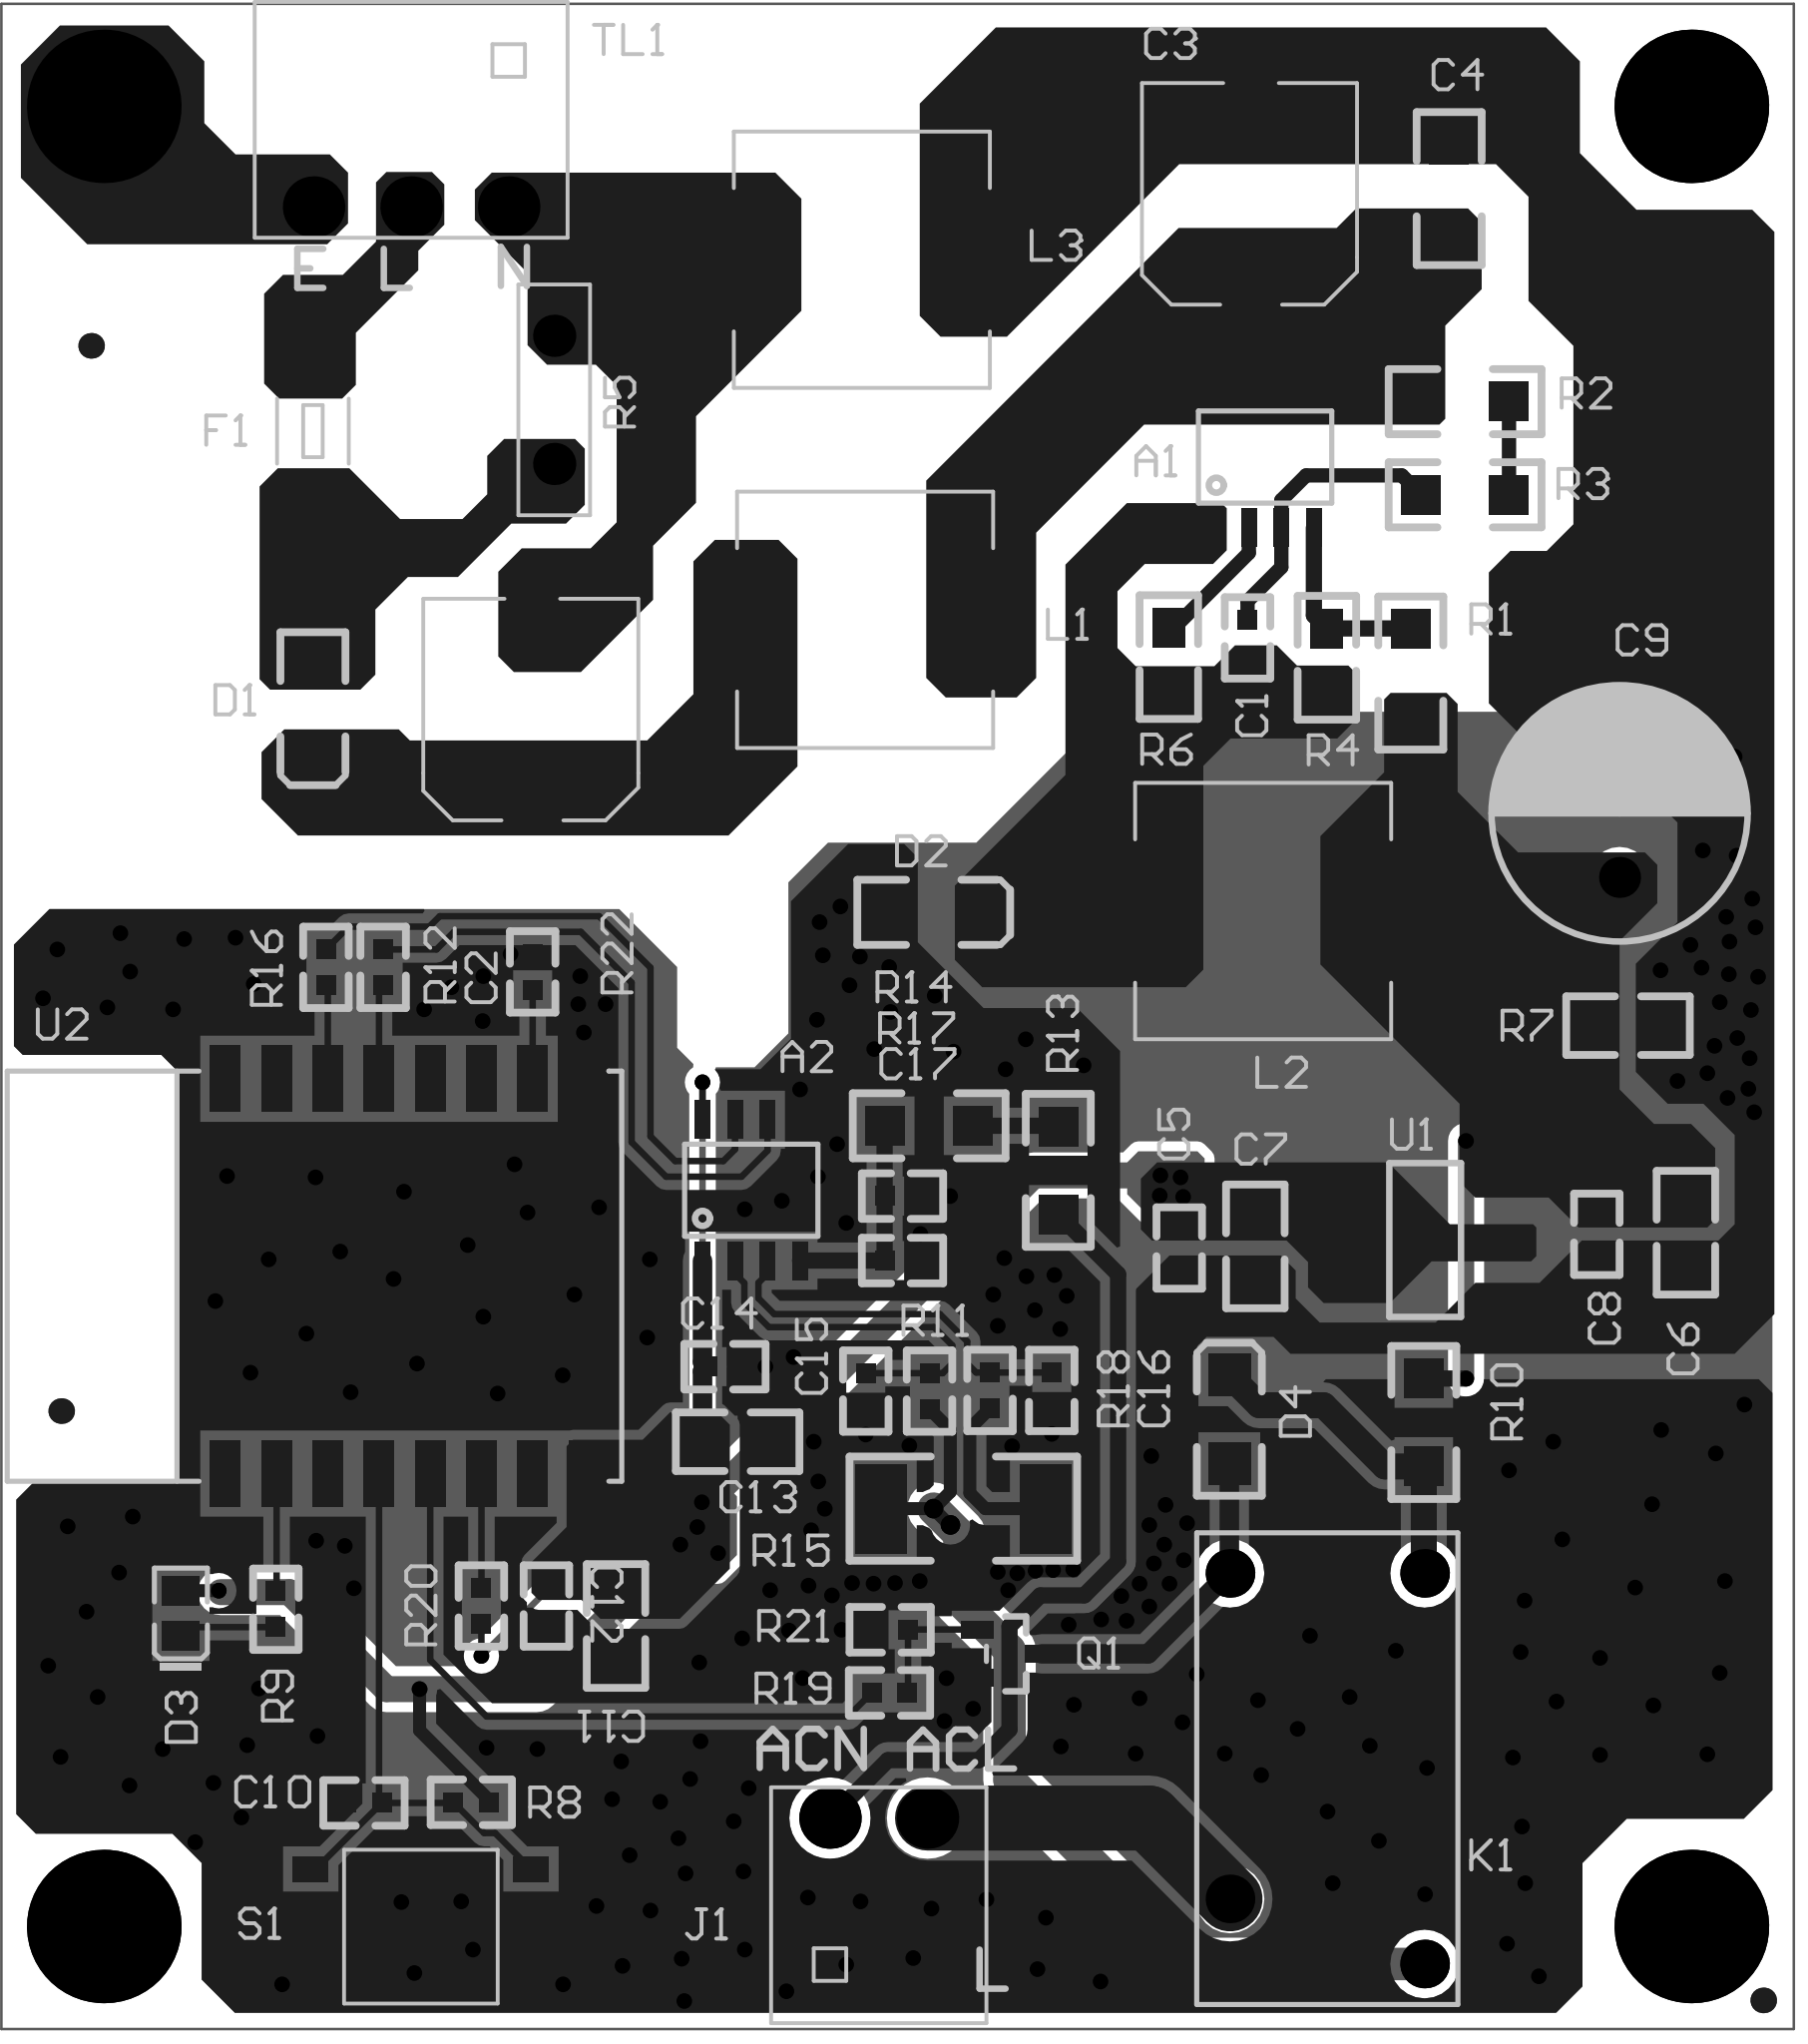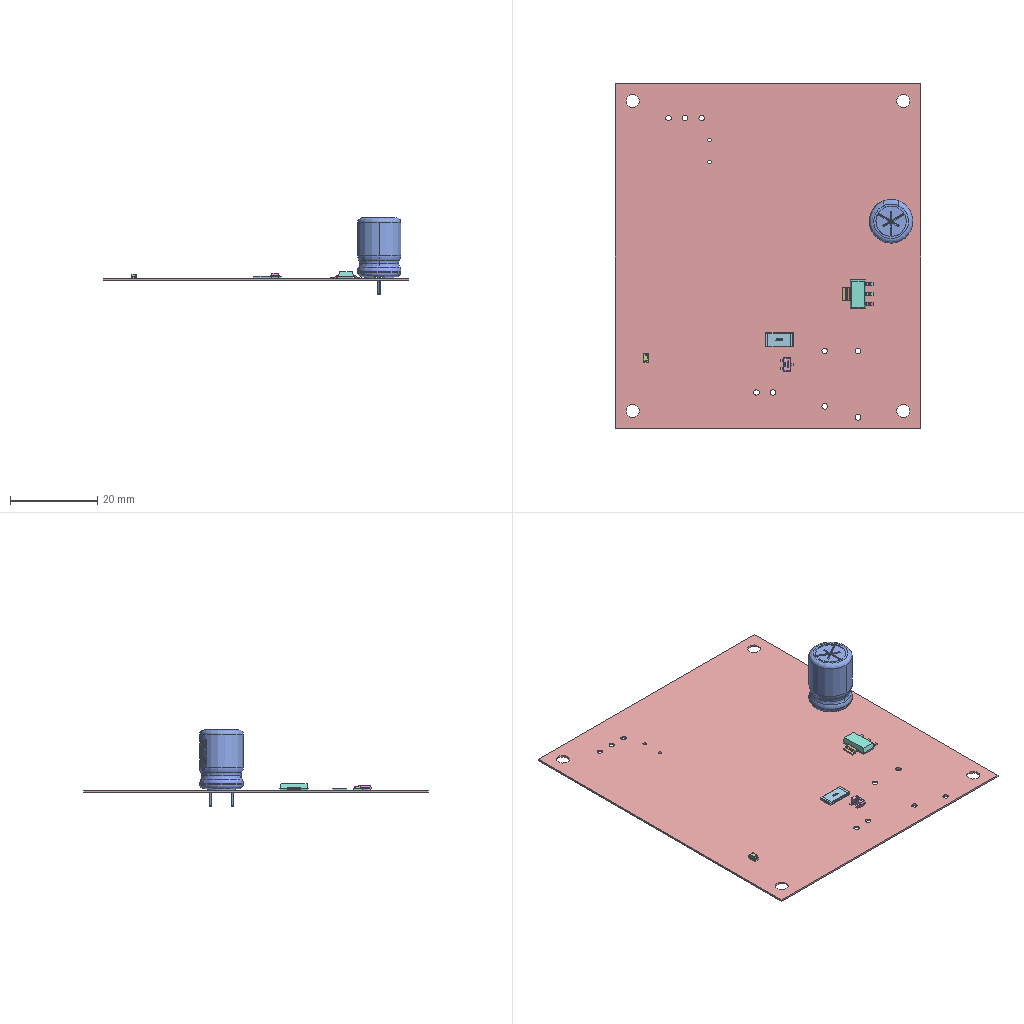Circuit board layout | Altium Designer | box 70 x 79 x 17.5 mm
Layer stack:
# Altium Designer layer stack of  (unit mm; dielectric type: 0 none, 1 core, 2 prepreg, 3 surface material)
index,name,kind,layer,copper_thickness_mm,dielectric_type,dielectric_thickness_mm,dielectric_material,dielectric_constant
0,Top Paste,other,,,,,,
1,Top Overlay,other,,,,,,
2,Top Solder,dielectric,,,3,0.0102,Solder Resist,3.5
3,Top Layer,copper,Top Layer,0.0356,,,,
4,Dielectric1,dielectric,,,0,0.32,FR-4,4.8
5,Bottom Layer,copper,Bottom Layer,0.0356,,,,
6,Bottom Solder,dielectric,,,3,0.0102,Solder Resist,3.5
7,Bottom Overlay,other,,,,,,
8,Bottom Paste,other,,,,,,
# drill layer pairs: low layer,high layer
drill_pair,Top Layer,Bottom Layer
Part placement:
Designator,Comment,Layer,Footprint,Center-X(mm),Center-Y(mm),Rotation
C6,10u/10V,TopLayer,0805,65.786,31.064,270
C7,10u/10V,TopLayer,0805,48.971,30.531,270
A1,SY50282,TopLayer,SO-8,49.352,61.321,90
A2,BL0937,TopLayer,SO-8,29.286,32.721,90
C1,2.2uF10% 50V,TopLayer,0603,48.666,54.267,270
C4,10nF10% 1kV,TopLayer,1206,56.54,71.793,90
C5,100nF (104) 10% 50V,TopLayer,0603,45.999,30.467,270
C8,100nF (104) 10% 50V,TopLayer,0603,62.306,31.001,270
C9,680u/16V,TopLayer,10X12.5,63.195,47.422,270
C10,100nF (104) 10% 50V,TopLayer,0603,14.161,8.82,180
C11,10u/10V,TopLayer,0805,24.003,15.723,270
C12,100nF (104) 10% 50V,TopLayer,0603,21.285,16.503,270
C13,10u/10V,TopLayer,0805,28.753,22.911,360
C14,100nF (104) 10% 50V,TopLayer,0603,28.258,25.838,360
C15,33nF 10% 50V,TopLayer,0603,33.757,24.885,270
C16,33nF 10% 50V,TopLayer,0603,41.021,24.91,90
C17,33nF 10% 50V,TopLayer,0603,35.192,29.978,360
D1,IN4007,TopLayer,SDIODE-2,12.167,51.504,90
D2,SS34,TopLayer,SDIODE-2,36.411,43.561,180
D3,Green 0805,TopLayer,0805_LED_S1,7.01,16.211,90
D4,IN4007,TopLayer,SDIODE-2,47.955,23.787,270
F1,MF2410F2.000TM,TopLayer,2410,12.167,62.332,270
J1,SIP2,TopLayer,DIP-2,34.265,8.23,360
K1,HF32F-G/005-HS3,TopLayer,HF32F-G/005-HS3,51.782,10.157,270
L1,VLP8040T-3R3N,TopLayer,IND10X10,33.731,54.971,180
L2,VLP8040T-3R3N,TopLayer,IND10X10,49.276,43.612,180
L3,VLP8040T-3R3N,TopLayer,IND10X10,33.604,69.018,180
Q1,S8050,TopLayer,SOT-23(SOT-23-3),39.37,14.636,180
R1,36K 1%,TopLayer,1206,55.042,52.895,90
R2,1.5M 1%,TopLayer,1206,57.163,63.48,360
R3,1.5M 1%,TopLayer,1206,57.163,59.848,180
R4,10K 1%,TopLayer,0805,51.765,53.492,270
R5,07d471K,TopLayer,07d471K,21.59,63.551,270
R6,0.9R 1%,TopLayer,0805,45.593,53.518,270
R7,3.3K 1%,TopLayer,0805,63.525,39.141,360
R8,10K,TopLayer,0603,18.352,8.845,180
R9,2K,TopLayer,0603,10.719,16.376,270
R10,330,TopLayer,1206,55.55,23.66,90
R11,1K 1%,TopLayer,0603,36.246,24.885,270
R12,100R1%,TopLayer,0603,14.91,41.415,270
R13,1M1%,TopLayer,1206,41.275,33.496,90
R14,1M1%,TopLayer,1206,36.233,35.236,180
R16,100R1%,TopLayer,0603,12.675,41.415,270
R17,1K 1%,TopLayer,0603,35.192,32.492,360
R18,1K 1%,TopLayer,0603,38.608,24.91,270
R19,2K,TopLayer,0603,34.684,13.112,180
R20,100R1%,TopLayer,0603,18.745,16.503,90
R21,10K,TopLayer,0603,34.709,15.576,180
S1,SW-PB4P,TopLayer,smd6X6x4.5,16.383,3.994,360
TL1,SIP3,TopLayer,DIP-3,16.002,71.075,180
U1,AMS1117-3.3,TopLayer,SOT-223,55.604,30.779,90
R15,1mR,TopLayer,2512,37.567,20.3,90
U2,WR3,TopLayer,WR3,15.748,29.368,90
R22,10K,TopLayer,0603,20.748,41.237,90
C2,3.3u/400V,TopLayer,SMD8x10.5,20.676,51.593,180
C3,3.3u/400V,TopLayer,SMD8x10.5,48.743,71.71,180
Pad and via stacks:
# Altium Designer via and pad stacks of  (unit mm). Each distinct definition once, with the count of objects using it.
# via: kind,start_layer,end_layer,hole_mm,diameter_mm,mode(0 simple;1 top-mid-bottom;2 full stack),diameter_per_layer,count,example_net
# pad: kind,layer,hole_mm,hole_type(0 round;1 square;2 slot),plating,top_size,top_shape(1 round;2 rect;3 octagon;9 rounded rect),mid_size,bottom_size,mode,footprint,size_per_layer,count,example
pad,Top Layer,0,0,plated,1x1,1,1x1,1x1,0,,,3,0
pad,Top Layer,0,0,plated,1.524x1.27,2,1.524x1.27,1.524x1.27,0,0805,,14,C6.1
pad,Top Layer,0,0,plated,0.762x0.762,2,0.762x0.762,0.762x0.762,0,0603,,40,R21.2
pad,Top Layer,0,0,plated,0.7x1.25,2,0.7x1.25,0.7x1.25,0,SOT-23(SOT-23-3),,3,Q1.1
pad,Top Layer,0,0,plated,1.651x1.651,2,1.651x1.651,1.651x1.651,0,SDIODE-2,,6,D4.A
pad,Top Layer,0,0,plated,1.16x1.47,2,1.16x1.47,1.16x1.47,0,0805_LED_S1,,2,D3.K
pad,Top Layer,0,0,plated,1.5x0.6,2,1.5x0.6,1.5x0.6,0,SO-8,,14,A2.1
pad,Top Layer,0,0,plated,1.5x0.5,2,1.5x0.5,1.5x0.5,0,SO-8,,2,A2.5
pad,Top Layer,0,0,plated,1x1.4,2,1x1.4,1x1.4,0,smd6X6x4.5,,4,S1.3
pad,Top Layer,0,0,plated,1.524x1.524,2,1.524x1.524,1.524x1.524,0,1206,,14,R10.2
pad,Top Layer,0,0,plated,5x3,2,5x3,5x3,0,IND10X10,,6,L3.1
pad,Top Layer,0,0,plated,3.5x2.2,2,3.5x2.2,3.5x2.2,0,SOT-223,,1,U1.2
pad,Top Layer,0,0,plated,1x2.2,2,1x2.2,1x2.2,0,SOT-223,,3,U1.3
pad,Top Layer,0,0,plated,2.6x2.6,2,2.6x2.6,2.6x2.6,0,2410,,2,F1.2
pad,Top Layer,0,0,plated,2x3.5,2,2x3.5,2x3.5,0,2512,,2,R15.1
pad,Top Layer,0,0,plated,1.2x2.6,2,1.2x2.6,1.2x2.6,0,WR3,,16,U2.16
pad,Top Layer,0,0,plated,3.2x1.6,2,3.2x1.6,3.2x1.6,0,SMD8x10.5,,4,C2.1
pad,Multi-Layer,3,0,plated,6x6,1,6x6,6x6,0,,,4,0
pad,Multi-Layer,1.3,0,plated,1.9x1.9,1,1.9x1.9,1.9x1.9,0,HF32F-G/005-HS3,,4,K1.1
pad,Multi-Layer,1.3,0,plated,2.4x2.4,1,2.4x2.4,2.4x2.4,0,DIP-2,,2,J1.2
pad,Multi-Layer,0.8,0,plated,1.65x1.65,1,1.65x1.65,1.65x1.65,0,07d471K,,2,R5.2
pad,Multi-Layer,1.3,0,plated,2.4x2.4,1,2.4x2.4,2.4x2.4,0,DIP-3,,3,TL1.1
pad,Multi-Layer,0.9,0,plated,1.6x1.6,1,1.6x1.6,1.6x1.6,0,10X12.5,,2,C9.1
pad,Bottom Layer,0,0,plated,1x1,1,1x1,1x1,0,,,3,0
via,Top Layer,Bottom Layer,0.3048,0.6096,0,,245,GND
via,Top Layer,Bottom Layer,0.381,0.762,0,,2,L_TO_R
Copper pours:
name,layer,net,type(0 solid;1 hatched;2 none)
Top Layer-No Net,Top Layer,+3.3V,0
Top Layer-No Net,Top Layer,+3.3V,0
Top Layer-No Net,Top Layer,+5V,0
Top Layer-No Net,Top Layer,GNDS,0
Top Layer-No Net,Top Layer,NetA1_5,0
Top Layer-No Net,Top Layer,NetC2_2,0
Top Layer-No Net,Top Layer,NetF1_1,0
Top Layer-No Net,Top Layer,NetD1_A,0
Top Layer-No Net,Top Layer,EARTH,0
Top Layer-No Net,Top Layer,NetC2_1,0
Top Layer-No Net,Top Layer,GND,0
Top Layer-No Net,Top Layer,GND,0
Top Layer-No Net,Bottom Layer,+3.3V,0
Top Layer-No Net,Bottom Layer,+3.3V,0
Top Layer-No Net,Bottom Layer,GND,0
Design rules, without the lines most boards share:
# Altium Designer design rules of  (exported by Altium Designer, unit mm)
# columns: name | kind | enabled | priority | scope1 | scope2 | descriptor | typed fields (field=value)
SilkToSilkClearance | 55 | enabled | 1 | All | All | Silk to Silk (Clearance=0mil) (All),(All) |
SilkToSolderMaskClearance | 54 | enabled | 1 | IsPad | All | Silk To Solder Mask (Clearance=0mil) (IsPad),(All) |
MinimumSolderMaskSliver | 53 | enabled | 1 | All | All | Minimum Solder Mask Sliver (Gap=0mil) (All),(All) |
HoleToHoleClearance | 52 | enabled | 1 | All | All | Hole To Hole Clearance (Gap=0mil) (All),(All) | gap=0
DiffPairsRouting | 51 | enabled | 1 | All | All | Differential Pairs Uncoupled Length using the Gap Constraints (Min=6.063mil) (Max=39.37mil) (Prefered=10mil)  and Width Constraints (Min=15mil) (Max=15mil) (Prefered=15mil) (All) |
HoleSize | 42 | enabled | 1 | All | All | Hole Size Constraint (Min=1mil) (Max=500mil) (All) |
SolderMaskExpansion | 13 | enabled | 1 | All | All | Solder Mask Expansion (Expansion =4mil) (All) | expansion=0.1016
PasteMaskExpansion | 14 | enabled | 1 | All | All | Paste Mask Expansion (Expansion =0mil) (All) | expansion=0
RoutingVias | 11 | enabled | 1 | All | All | Routing Via (MinHoleWidth=12mil) (MaxHoleWidth=12mil) (PreferredHoleWidth=12mil) (MinWidth=24mil) (MaxWidth=24mil) (PreferedWidth=24mil) (All) | via_min_hole=0.3048 via_max_hole=0.3048 via_preferred_diameter=0.6096 via_preferred_hole=0.3048
Width | 2 | enabled | 1 | All | All | Width Constraint (Min=10mil) (Max=100mil) (Preferred=10mil) (All) |
PolygonConnect | 20 | enabled | 2 | All | All | Polygon Connect Rule(Direct Connect )(Conductor Width=20mil) (Relief Angle=90 Angle) (Entries=4) (Air Gap Width=10mil) (All),(All) | connect_style(0=relief,1=direct,2=none)=1 relief_conductor_width=0.508 relief_entries=4
PlaneConnect | 6 | enabled | 1 | All | All | Power Plane Connect Rule(Relief Connect )(Expansion=20mil) (Conductor Width=19.685mil) (Air Gap=10mil) (Entries=4) (All) | relief_conductor_width=0.5 relief_entries=4 relief_expansion=0.508
Clearance | 0 | enabled | 2 | All | All | Clearance Constraint (Gap=10mil) (All),(All) | gap=0.254
Clearance_1 | 0 | enabled | 1 | INPOLYGON | All | Clearance Constraint (Gap=10mil) (INPOLYGON),(All) | gap=0.254
PolygonConnect_1 | 20 | enabled | 1 | All | ISVIA | Polygon Connect Rule(Direct Connect )(Conductor Width=10mil) (Relief Angle=90 Angle) (Entries=4) (Air Gap Width=10mil) (All),(ISVIA) | connect_style(0=relief,1=direct,2=none)=1 relief_conductor_width=0.254 relief_entries=4
Classes set for this board:
# Altium Designer classes of  (member kind: 0 net, 1 component, 2 from-to, 3 pad, 4 layer, 5 differential pair, 6 design channel, 7 polygon, 8 structure, 9 xSignal)
# columns: class name | member kind | superclass | members
WIFI | 1 | no | C11; C12; CF134; CF135; CF136; CF137; CF138; CF139; CF148; CF149; CF150; CF151; CF152; CF153; D2; D1; D3; K1; LF12; LF13; Q1; R6; R5; R3; R4; R1; U2; C38; C65; K1; R54; R55; R112; R113; R114; R115; U1; C38; C65; K1; R54; R55; R112; R113; R114; R115; J1; U1; J1; C4; C3; K1; C6; C7; C8; C9; C12; C16; C17; D4; L1; R2; R7; R8; R9; R10; R11; R12; R13; R14; R15; R16; R17; R18; R19; R20; R21; U2; C5; C10; S1; C11; A1; A2; C13; C14; C15; F1; L2; L3; TL1; C1; C2; U1; A1; A2; C1; C2; C3; C4; C5; C8; C9; C10; C11; C12; C13; C14; C15; C16; C17; D1; D2; D3; D4; F1; J1; K1; L1; L2; L3; Q1; R1; R2; R3; R4; R5; R6; R7; R8; R9; R10; R11; R12; R13; R14; R16; R17; R18; R19; R20; R21; S1; TL1; U1; U2; R15; U2; R22; C2; C3;